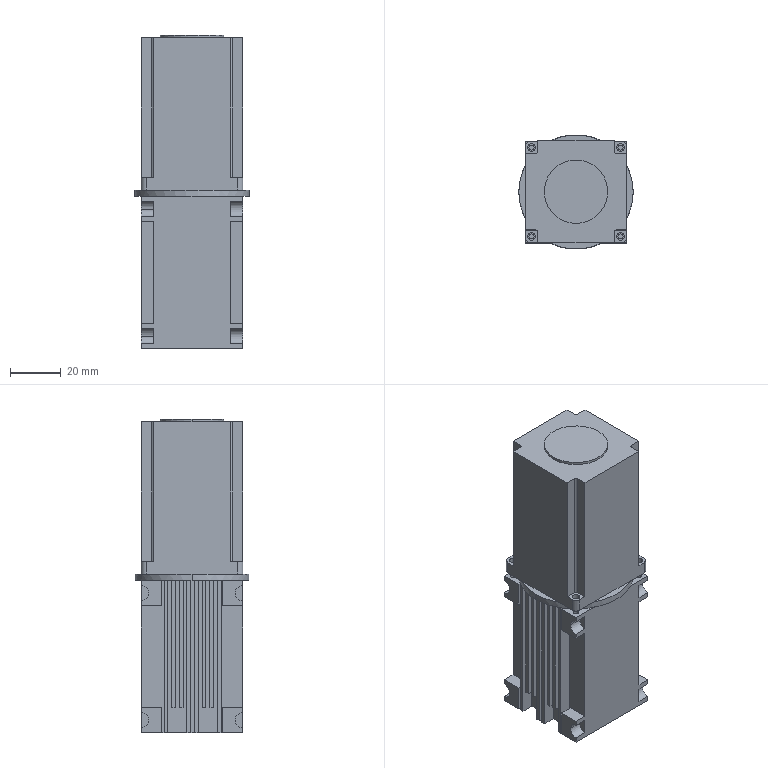Part | SolidWorks | 2 solids | 190 faces | box 45 x 45 x 123.5 mm | volume 175871 mm3 | plane 144 | cylinder 46 | commonest cylinder face diameters 2 x12 6 x12 3 x8 4 x4 10 x4 5 x2